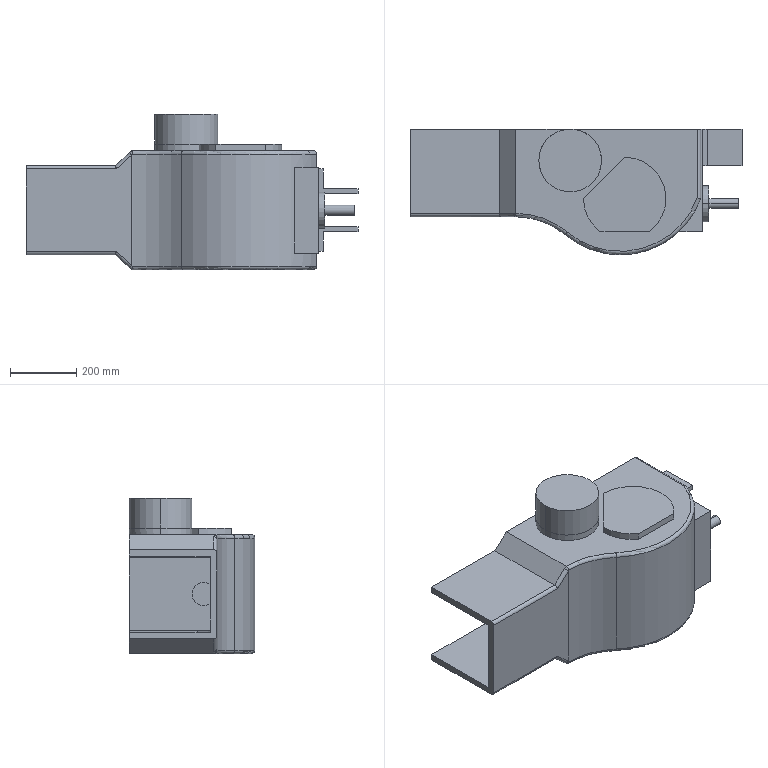Part | SolidWorks | 1 solid | 76 faces | box 1005 x 380.05 x 470 mm | volume 23114578 mm3 | plane 48 | cylinder 22 | torus 4 | spline 2 | commonest cylinder face diameters 20 x6 30 x2 70 x2 110 x2 190 x2 190.1 x2